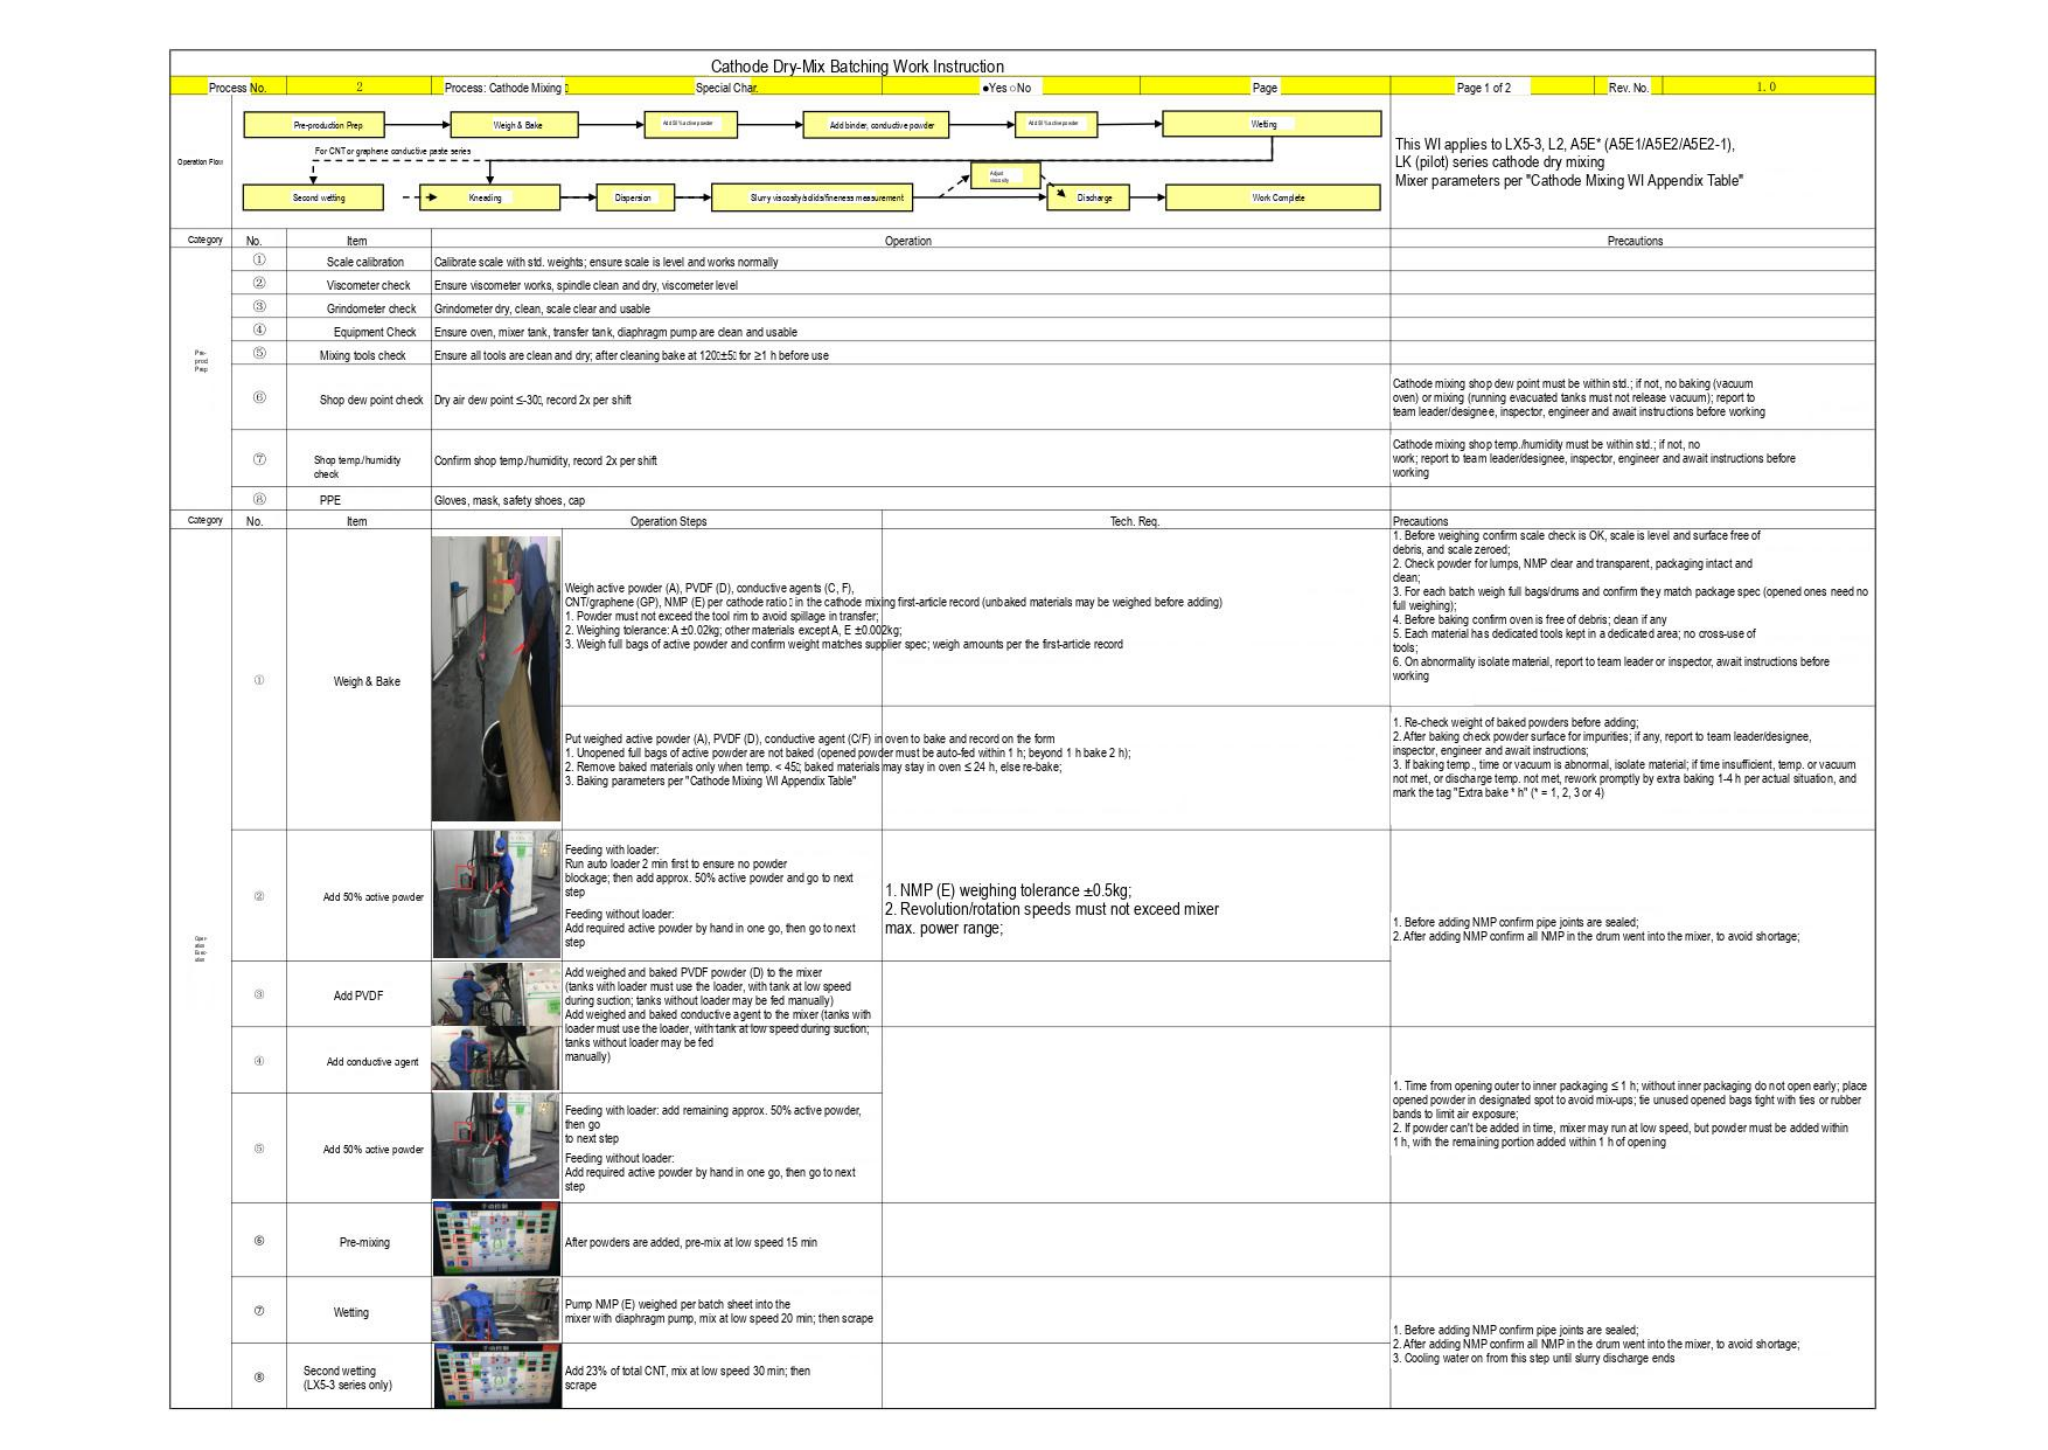# Cathode Dry-Mix Batching Work Instruction

| Process No. | 2 | Process: Cathode Mixing □ | Special Char. | ●Yes ○No | Page | Page 1 of 2 | Rev. No. | 1.0 |
|---|---|---|---|---|---|---|---|---|

Operation Flow

Pre-production Prep → Weigh & Bake → Add 50% active powder → Add binder, conductive powder → Add 50% active powder → Wetting

For CNT or graphene conductive paste series

Second wetting → Kneading → Dispersion → Slurry viscosity/solids/fineness measurement → Adjust viscosity → Discharge → Work Complete

This WI applies to LX5-3, L2, A5E* (A5E1/A5E2/A5E2-1), LK (pilot) series cathode dry mixing
Mixer parameters per "Cathode Mixing WI Appendix Table"

| Category | No. | Item | Operation | Precautions |
|---|---|---|---|---|
| Pre-prod Prep | ① | Scale calibration | Calibrate scale with std. weights; ensure scale is level and works normally | |
| | ② | Viscometer check | Ensure viscometer works, spindle clean and dry, viscometer level | |
| | ③ | Grindometer check | Grindometer dry, clean, scale clear and usable | |
| | ④ | Equipment Check | Ensure oven, mixer tank, transfer tank, diaphragm pump are clean and usable | |
| | ⑤ | Mixing tools check | Ensure all tools are clean and dry; after cleaning bake at 120□±5□ for ≥1 h before use | |
| | ⑥ | Shop dew point check | Dry air dew point ≤-30□, record 2x per shift | Cathode mixing shop dew point must be within std.; if not, no baking (vacuum oven) or mixing (running evacuated tanks must not release vacuum); report to team leader/designee, inspector, engineer and await instructions before working |
| | ⑦ | Shop temp./humidity check | Confirm shop temp./humidity, record 2x per shift | Cathode mixing shop temp./humidity must be within std.; if not, no work; report to team leader/designee, inspector, engineer and await instructions before working |
| | ⑧ | PPE | Gloves, mask, safety shoes, cap | |

| Category | No. | Item | Operation Steps | Tech. Req. | Precautions |
|---|---|---|---|---|---|
| Operation Execution | ① | Weigh & Bake | Weigh active powder (A), PVDF (D), conductive agents (C, F), CNT/graphene (GP), NMP (E) per cathode ratio□ in the cathode mixing first-article record (unbaked materials may be weighed before adding)<br>1. Powder must not exceed the tool rim to avoid spillage in transfer;<br>2. Weighing tolerance: A ±0.02kg; other materials except A, E ±0.002kg;<br>3. Weigh full bags of active powder and confirm weight matches supplier spec; weigh amounts per the first-article record | | 1. Before weighing confirm scale check is OK, scale is level and surface free of debris, and scale zeroed;<br>2. Check powder for lumps, NMP clear and transparent, packaging intact and clean;<br>3. For each batch weigh full bags/drums and confirm they match package spec (opened ones need no full weighing);<br>4. Before baking confirm oven is free of debris; clean if any<br>5. Each material has dedicated tools kept in a dedicated area; no cross-use of tools;<br>6. On abnormality isolate material, report to team leader or inspector, await instructions before working |
| | | | Put weighed active powder (A), PVDF (D), conductive agent (C/F) in oven to bake and record on the form<br>1. Unopened full bags of active powder are not baked (opened powder must be auto-fed within 1 h; beyond 1 h bake 2 h);<br>2. Remove baked materials only when temp. < 45□; baked materials may stay in oven ≤ 24 h, else re-bake;<br>3. Baking parameters per "Cathode Mixing WI Appendix Table" | | 1. Re-check weight of baked powders before adding;<br>2. After baking check powder surface for impurities; if any, report to team leader/designee, inspector, engineer and await instructions;<br>3. If baking temp., time or vacuum is abnormal, isolate material; if time insufficient, temp. or vacuum not met, or discharge temp. not met, rework promptly by extra baking 1-4 h per actual situation, and mark the tag "Extra bake * h" (* = 1, 2, 3 or 4) |
| | ② | Add 50% active powder | Feeding with loader:<br>Run auto loader 2 min first to ensure no powder blockage; then add approx. 50% active powder and go to next step<br>Feeding without loader:<br>Add required active powder by hand in one go, then go to next step | 1. NMP (E) weighing tolerance ±0.5kg;<br>2. Revolution/rotation speeds must not exceed mixer max. power range; | 1. Before adding NMP confirm pipe joints are sealed;<br>2. After adding NMP confirm all NMP in the drum went into the mixer, to avoid shortage; |
| | ③ | Add PVDF | Add weighed and baked PVDF powder (D) to the mixer (tanks with loader must use the loader, with tank at low speed during suction; tanks without loader may be fed manually) | | |
| | ④ | Add conductive agent | Add weighed and baked conductive agent to the mixer (tanks with loader must use the loader, with tank at low speed during suction; tanks without loader may be fed manually) | | 1. Time from opening outer to inner packaging ≤ 1 h; without inner packaging do not open early; place opened powder in designated spot to avoid mix-ups; tie unused opened bags tight with ties or rubber bands to limit air exposure;<br>2. If powder can't be added in time, mixer may run at low speed, but powder must be added within 1 h, with the remaining portion added within 1 h of opening |
| | ⑤ | Add 50% active powder | Feeding with loader: add remaining approx. 50% active powder, then go to next step<br>Feeding without loader:<br>Add required active powder by hand in one go, then go to next step | | |
| | ⑥ | Pre-mixing | After powders are added, pre-mix at low speed 15 min | | |
| | ⑦ | Wetting | Pump NMP (E) weighed per batch sheet into the mixer with diaphragm pump, mix at low speed 20 min; then scrape | | 1. Before adding NMP confirm pipe joints are sealed;<br>2. After adding NMP confirm all NMP in the drum went into the mixer, to avoid shortage;<br>3. Cooling water on from this step until slurry discharge ends |
| | ⑧ | Second wetting (LX5-3 series only) | Add 23% of total CNT, mix at low speed 30 min; then scrape | | |
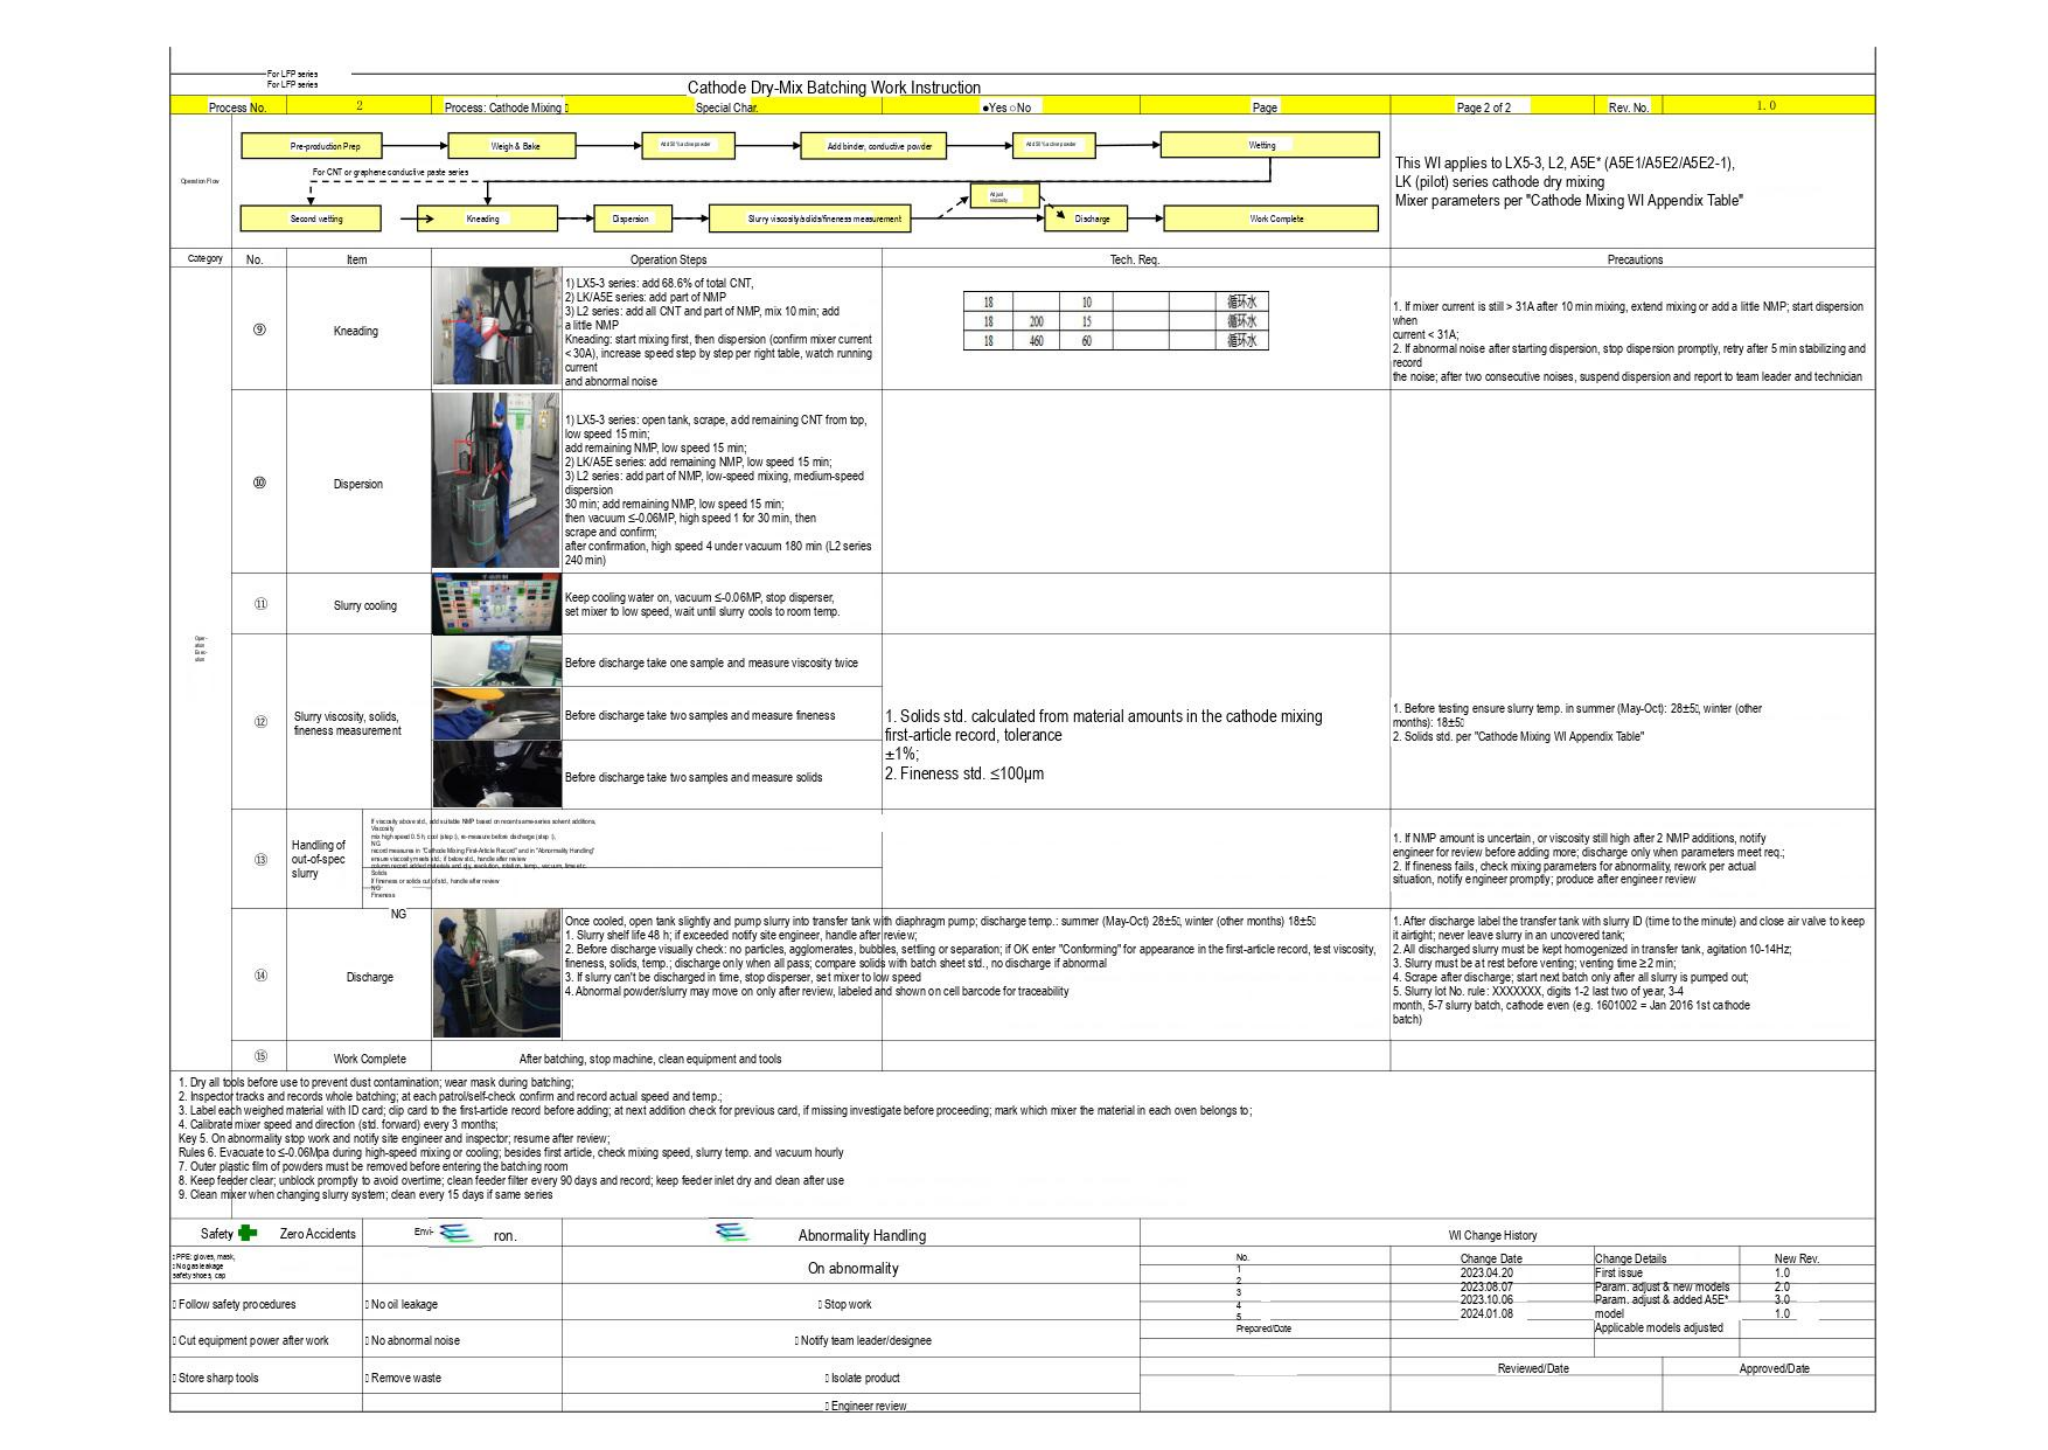For LFP series
For LFP series

# Cathode Dry-Mix Batching Work Instruction

| Process No. | 2 | Process: Cathode Mixing | Special Char. | ●Yes ○No | Page | Page 2 of 2 | Rev. No. | 1.0 |
|---|---|---|---|---|---|---|---|---|

Operation Flow

Pre-production Prep → Weigh & Bake → Add 50% active powder → Add binder, conductive powder → Add 50% active powder → Wetting

For CNT or graphene conductive paste series

Second wetting → Kneading → Dispersion → Slurry viscosity/solids/fineness measurement → Adjust viscosity → Discharge → Work Complete

This WI applies to LX5-3, L2, A5E* (A5E1/A5E2/A5E2-1), LK (pilot) series cathode dry mixing
Mixer parameters per "Cathode Mixing WI Appendix Table"

| Category | No. | Item | Operation Steps | Tech. Req. | Precautions |
|---|---|---|---|---|---|
| Operation Execution | ⑨ | Kneading | 1) LX5-3 series: add 68.6% of total CNT,<br>2) LK/A5E series: add part of NMP<br>3) L2 series: add all CNT and part of NMP, mix 10 min; add a little NMP<br>Kneading: start mixing first, then dispersion (confirm mixer current < 30A), increase speed step by step per right table, watch running current and abnormal noise | 18 \| \| 10 \| \| \| 循环水<br>18 \| 200 \| 15 \| \| \| 循环水<br>18 \| 460 \| 60 \| \| \| 循环水 | 1. If mixer current is still > 31A after 10 min mixing, extend mixing or add a little NMP; start dispersion when current < 31A;<br>2. If abnormal noise after starting dispersion, stop dispersion promptly, retry after 5 min stabilizing and record the noise; after two consecutive noises, suspend dispersion and report to team leader and technician |
| | ⑩ | Dispersion | 1) LX5-3 series: open tank, scrape, add remaining CNT from top, low speed 15 min;<br>add remaining NMP, low speed 15 min;<br>2) LK/A5E series: add remaining NMP, low speed 15 min;<br>3) L2 series: add part of NMP, low-speed mixing, medium-speed dispersion 30 min; add remaining NMP, low speed 15 min;<br>then vacuum ≤-0.06MP, high speed 1 for 30 min, then scrape and confirm;<br>after confirmation, high speed 4 under vacuum 180 min (L2 series 240 min) | | |
| | ⑪ | Slurry cooling | Keep cooling water on, vacuum ≤-0.06MP, stop disperser, set mixer to low speed, wait until slurry cools to room temp. | | |
| | ⑫ | Slurry viscosity, solids, fineness measurement | Before discharge take one sample and measure viscosity twice<br>Before discharge take two samples and measure fineness<br>Before discharge take two samples and measure solids | 1. Solids std. calculated from material amounts in the cathode mixing first-article record, tolerance ±1%;<br>2. Fineness std. ≤100μm | 1. Before testing ensure slurry temp. in summer (May-Oct): 28±5; winter (other months): 18±5<br>2. Solids std. per "Cathode Mixing WI Appendix Table" |
| | ⑬ | Handling of out-of-spec slurry | Viscosity: If viscosity above std., add suitable NMP based on recent same-series solvent additions, mix high speed 0.5 h, cool (step ), re-measure before discharge (step ), record measures in "Cathode Mixing First-Article Record" and in "Abnormality Handling"; ensure viscosity meets std.; if below std., handle after review; column record added materials and qty, resolution, rotation, temp., vacuum, time etc. NG<br>Solids / Fineness: If fineness or solids out of std., handle after review NG<br>NG | | 1. If NMP amount is uncertain, or viscosity still high after 2 NMP additions, notify engineer for review before adding more; discharge only when parameters meet req.;<br>2. If fineness fails, check mixing parameters for abnormality, rework per actual situation, notify engineer promptly; produce after engineer review |
| | ⑭ | Discharge | Once cooled, open tank slightly and pump slurry into transfer tank with diaphragm pump; discharge temp.: summer (May-Oct) 28±5; winter (other months) 18±5<br>1. Slurry shelf life 48 h; if exceeded notify site engineer, handle after review;<br>2. Before discharge visually check: no particles, agglomerates, bubbles, settling or separation; if OK enter "Conforming" for appearance in the first-article record, test viscosity, fineness, solids, temp.; discharge only when all pass; compare solids with batch sheet std., no discharge if abnormal<br>3. If slurry can't be discharged in time, stop disperser, set mixer to low speed<br>4. Abnormal powder/slurry may move on only after review, labeled and shown on cell barcode for traceability | | 1. After discharge label the transfer tank with slurry ID (time to the minute) and close air valve to keep it airtight; never leave slurry in an uncovered tank;<br>2. All discharged slurry must be kept homogenized in transfer tank, agitation 10-14Hz;<br>3. Slurry must be at rest before venting; venting time ≥2 min;<br>4. Scrape after discharge; start next batch only after all slurry is pumped out;<br>5. Slurry lot No. rule: XXXXXXX, digits 1-2 last two of year, 3-4 month, 5-7 slurry batch, cathode even (e.g. 1601002 = Jan 2016 1st cathode batch) |
| | ⑮ | Work Complete | After batching, stop machine, clean equipment and tools | | |

Key Rules
1. Dry all tools before use to prevent dust contamination; wear mask during batching;
2. Inspector tracks and records whole batching; at each patrol/self-check confirm and record actual speed and temp.;
3. Label each weighed material with ID card; clip card to the first-article record before adding; at next addition check for previous card, if missing investigate before proceeding; mark which mixer the material in each oven belongs to;
4. Calibrate mixer speed and direction (std. forward) every 3 months;
5. On abnormality stop work and notify site engineer and inspector; resume after review;
6. Evacuate to ≤-0.06Mpa during high-speed mixing or cooling; besides first article, check mixing speed, slurry temp. and vacuum hourly
7. Outer plastic film of powders must be removed before entering the batching room
8. Keep feeder clear; unblock promptly to avoid overtime; clean feeder filter every 90 days and record; keep feeder inlet dry and clean after use
9. Clean mixer when changing slurry system; clean every 15 days if same series

| Safety Zero Accidents | Envi-ron. | Abnormality Handling |
|---|---|---|
| PPE: gloves, mask, safety shoes, cap<br>No gas leakage | | On abnormality |
| Follow safety procedures | No oil leakage | Stop work |
| Cut equipment power after work | No abnormal noise | Notify team leader/designee |
| Store sharp tools | Remove waste | Isolate product |
| | | Engineer review |

WI Change History

| No. | Change Date | Change Details | New Rev. |
|---|---|---|---|
| 1 | 2023.04.20 | First issue | 1.0 |
| 2 | 2023.08.07 | Param. adjust & new models | 2.0 |
| 3 | 2023.10.06 | Param. adjust & added A5E* model | 3.0 |
| 4 | 2024.01.08 | Applicable models adjusted | 1.0 |
| 5 | | | |

| Prepared/Date | Reviewed/Date | Approved/Date |
|---|---|---|
| | | |